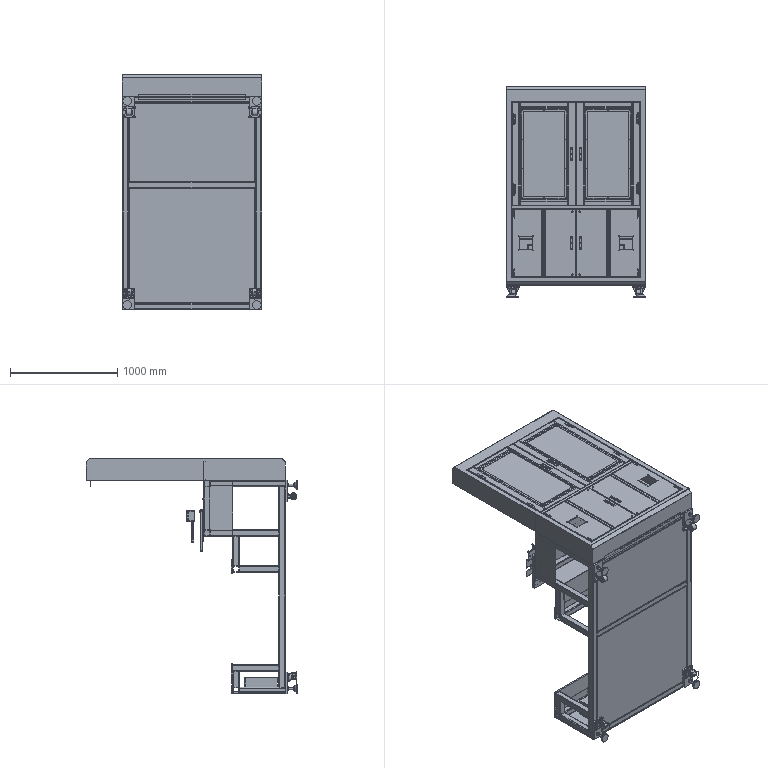Part | NX | features BREP 79 | 125 solids | 5196 faces | volume 59659236 mm3 | plane 2185 | cylinder 2073 | cone 502 | torus 324 | spline 112 | commonest cylinder face diameters 5 x324 8 x184 7 x182 4 x162 6 x160 16 x120